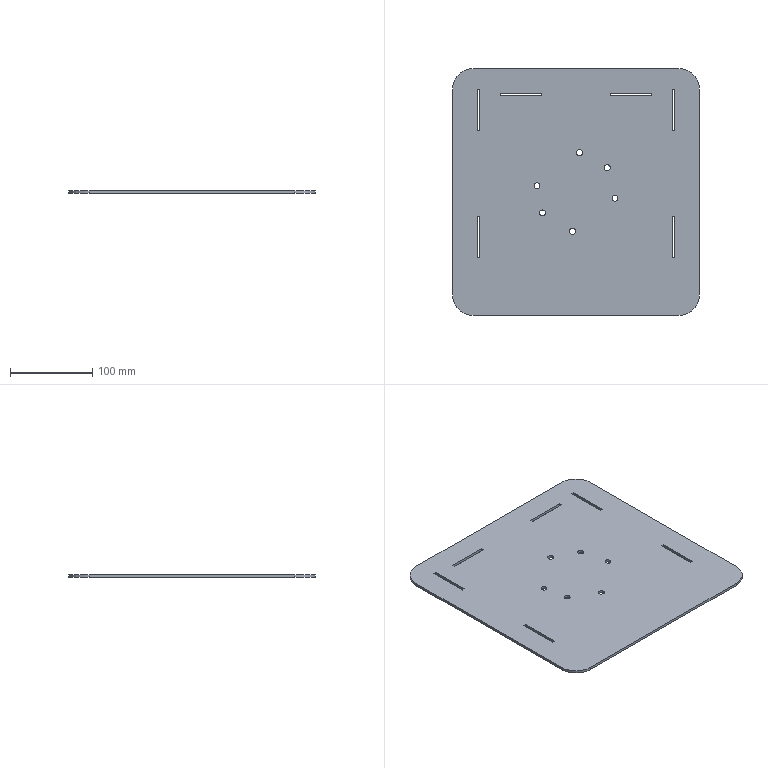Part | SolidWorks | features FlatPattern 1, SMBaseFlange 1, SheetMetal 1 | 1 solid | 46 faces | box 300 x 300 x 3.2 mm | volume 282429 mm3 | plane 30 | cylinder 16 | commonest cylinder face diameters 7.2 x12 50 x4
STEP:
#1=CARTESIAN_POINT('',(-41.465,31.655,3.2));
#2=VERTEX_POINT('',#1);
#3=CARTESIAN_POINT('',(-34.265,31.655,3.2));
#4=VERTEX_POINT('',#3);
#5=CARTESIAN_POINT('',(-37.865,31.655,3.2));
#6=DIRECTION('',(0.,0.,1.));
#7=DIRECTION('',(1.,0.,0.));
#8=AXIS2_PLACEMENT_3D('',#5,#6,#7);
#9=CIRCLE('',#8,3.6);
#10=EDGE_CURVE('',#2,#4,#9,.T.);
#11=ORIENTED_EDGE('',*,*,#10,.T.);
#12=CARTESIAN_POINT('',(-34.265,31.655,0.));
#13=VERTEX_POINT('',#12);
#14=CARTESIAN_POINT('',(-34.265,31.655,3.2));
#15=DIRECTION('',(0.,0.,-1.));
#16=VECTOR('',#15,1000.);
#17=LINE('',#14,#16);
#18=EDGE_CURVE('',#4,#13,#17,.T.);
#19=ORIENTED_EDGE('',*,*,#18,.T.);
#20=CARTESIAN_POINT('',(-41.465,31.655,0.));
#21=VERTEX_POINT('',#20);
#22=CARTESIAN_POINT('',(-37.865,31.655,0.));
#23=DIRECTION('',(0.,0.,1.));
#24=DIRECTION('',(1.,0.,0.));
#25=AXIS2_PLACEMENT_3D('',#22,#23,#24);
#26=CIRCLE('',#25,3.6);
#27=EDGE_CURVE('',#21,#13,#26,.T.);
#28=ORIENTED_EDGE('',*,*,#27,.F.);
#29=CARTESIAN_POINT('',(-41.465,31.655,3.2));
#30=DIRECTION('',(0.,0.,-1.));
#31=VECTOR('',#30,1000.);
#32=LINE('',#29,#31);
#33=EDGE_CURVE('',#2,#21,#32,.T.);
#34=ORIENTED_EDGE('',*,*,#33,.F.);
#35=EDGE_LOOP('',(#11,#19,#28,#34));
#36=FACE_OUTER_BOUND('',#35,.T.);
#37=CARTESIAN_POINT('',(-37.865,31.655,3.2));
#38=DIRECTION('',(0.,0.,-1.));
#39=DIRECTION('',(-1.,0.,0.));
#40=AXIS2_PLACEMENT_3D('',#37,#38,#39);
#41=CYLINDRICAL_SURFACE('',#40,3.6);
#42=ADVANCED_FACE('',(#36),#41,.F.);
#43=CARTESIAN_POINT('',(-34.762,-1.29,3.2));
#44=VERTEX_POINT('',#43);
#45=CARTESIAN_POINT('',(-27.562,-1.29,3.2));
#46=VERTEX_POINT('',#45);
#47=CARTESIAN_POINT('',(-31.162,-1.29,3.2));
#48=DIRECTION('',(0.,0.,1.));
#49=DIRECTION('',(1.,0.,0.));
#50=AXIS2_PLACEMENT_3D('',#47,#48,#49);
#51=CIRCLE('',#50,3.6);
#52=EDGE_CURVE('',#44,#46,#51,.T.);
#53=ORIENTED_EDGE('',*,*,#52,.T.);
#54=CARTESIAN_POINT('',(-27.562,-1.29,0.));
#55=VERTEX_POINT('',#54);
#56=CARTESIAN_POINT('',(-27.562,-1.29,3.2));
#57=DIRECTION('',(0.,0.,-1.));
#58=VECTOR('',#57,1000.);
#59=LINE('',#56,#58);
#60=EDGE_CURVE('',#46,#55,#59,.T.);
#61=ORIENTED_EDGE('',*,*,#60,.T.);
#62=CARTESIAN_POINT('',(-34.762,-1.29,0.));
#63=VERTEX_POINT('',#62);
#64=CARTESIAN_POINT('',(-31.162,-1.29,0.));
#65=DIRECTION('',(0.,0.,1.));
#66=DIRECTION('',(1.,0.,0.));
#67=AXIS2_PLACEMENT_3D('',#64,#65,#66);
#68=CIRCLE('',#67,3.6);
#69=EDGE_CURVE('',#63,#55,#68,.T.);
#70=ORIENTED_EDGE('',*,*,#69,.F.);
#71=CARTESIAN_POINT('',(-34.762,-1.29,3.2));
#72=DIRECTION('',(0.,0.,-1.));
#73=VECTOR('',#72,1000.);
#74=LINE('',#71,#73);
#75=EDGE_CURVE('',#44,#63,#74,.T.);
#76=ORIENTED_EDGE('',*,*,#75,.F.);
#77=EDGE_LOOP('',(#53,#61,#70,#76));
#78=FACE_OUTER_BOUND('',#77,.T.);
#79=CARTESIAN_POINT('',(-31.162,-1.29,3.2));
#80=DIRECTION('',(0.,0.,-1.));
#81=DIRECTION('',(-1.,0.,0.));
#82=AXIS2_PLACEMENT_3D('',#79,#80,#81);
#83=CYLINDRICAL_SURFACE('',#82,3.6);
#84=ADVANCED_FACE('',(#78),#83,.F.);
#85=CARTESIAN_POINT('',(1.761,-23.671,3.2));
#86=VERTEX_POINT('',#85);
#87=CARTESIAN_POINT('',(8.961,-23.671,3.2));
#88=VERTEX_POINT('',#87);
#89=CARTESIAN_POINT('',(5.361,-23.671,3.2));
#90=DIRECTION('',(0.,0.,1.));
#91=DIRECTION('',(1.,0.,0.));
#92=AXIS2_PLACEMENT_3D('',#89,#90,#91);
#93=CIRCLE('',#92,3.6);
#94=EDGE_CURVE('',#86,#88,#93,.T.);
#95=ORIENTED_EDGE('',*,*,#94,.T.);
#96=CARTESIAN_POINT('',(8.961,-23.671,0.));
#97=VERTEX_POINT('',#96);
#98=CARTESIAN_POINT('',(8.961,-23.671,3.2));
#99=DIRECTION('',(0.,0.,-1.));
#100=VECTOR('',#99,1000.);
#101=LINE('',#98,#100);
#102=EDGE_CURVE('',#88,#97,#101,.T.);
#103=ORIENTED_EDGE('',*,*,#102,.T.);
#104=CARTESIAN_POINT('',(1.761,-23.671,0.));
#105=VERTEX_POINT('',#104);
#106=CARTESIAN_POINT('',(5.361,-23.671,0.));
#107=DIRECTION('',(0.,0.,1.));
#108=DIRECTION('',(1.,0.,0.));
#109=AXIS2_PLACEMENT_3D('',#106,#107,#108);
#110=CIRCLE('',#109,3.6);
#111=EDGE_CURVE('',#105,#97,#110,.T.);
#112=ORIENTED_EDGE('',*,*,#111,.F.);
#113=CARTESIAN_POINT('',(1.761,-23.671,3.2));
#114=DIRECTION('',(0.,0.,-1.));
#115=VECTOR('',#114,1000.);
#116=LINE('',#113,#115);
#117=EDGE_CURVE('',#86,#105,#116,.T.);
#118=ORIENTED_EDGE('',*,*,#117,.F.);
#119=EDGE_LOOP('',(#95,#103,#112,#118));
#120=FACE_OUTER_BOUND('',#119,.T.);
#121=CARTESIAN_POINT('',(5.361,-23.671,3.2));
#122=DIRECTION('',(0.,0.,-1.));
#123=DIRECTION('',(-1.,0.,0.));
#124=AXIS2_PLACEMENT_3D('',#121,#122,#123);
#125=CYLINDRICAL_SURFACE('',#124,3.6);
#126=ADVANCED_FACE('',(#120),#125,.F.);
#127=CARTESIAN_POINT('',(53.354,16.637,3.2));
#128=VERTEX_POINT('',#127);
#129=CARTESIAN_POINT('',(60.554,16.637,3.2));
#130=VERTEX_POINT('',#129);
#131=CARTESIAN_POINT('',(56.954,16.637,3.2));
#132=DIRECTION('',(0.,0.,1.));
#133=DIRECTION('',(1.,0.,0.));
#134=AXIS2_PLACEMENT_3D('',#131,#132,#133);
#135=CIRCLE('',#134,3.6);
#136=EDGE_CURVE('',#128,#130,#135,.T.);
#137=ORIENTED_EDGE('',*,*,#136,.T.);
#138=CARTESIAN_POINT('',(60.554,16.637,0.));
#139=VERTEX_POINT('',#138);
#140=CARTESIAN_POINT('',(60.554,16.637,3.2));
#141=DIRECTION('',(0.,0.,-1.));
#142=VECTOR('',#141,1000.);
#143=LINE('',#140,#142);
#144=EDGE_CURVE('',#130,#139,#143,.T.);
#145=ORIENTED_EDGE('',*,*,#144,.T.);
#146=CARTESIAN_POINT('',(53.354,16.637,0.));
#147=VERTEX_POINT('',#146);
#148=CARTESIAN_POINT('',(56.954,16.637,0.));
#149=DIRECTION('',(0.,0.,1.));
#150=DIRECTION('',(1.,0.,0.));
#151=AXIS2_PLACEMENT_3D('',#148,#149,#150);
#152=CIRCLE('',#151,3.6);
#153=EDGE_CURVE('',#147,#139,#152,.T.);
#154=ORIENTED_EDGE('',*,*,#153,.F.);
#155=CARTESIAN_POINT('',(53.354,16.637,3.2));
#156=DIRECTION('',(0.,0.,-1.));
#157=VECTOR('',#156,1000.);
#158=LINE('',#155,#157);
#159=EDGE_CURVE('',#128,#147,#158,.T.);
#160=ORIENTED_EDGE('',*,*,#159,.F.);
#161=EDGE_LOOP('',(#137,#145,#154,#160));
#162=FACE_OUTER_BOUND('',#161,.T.);
#163=CARTESIAN_POINT('',(56.954,16.637,3.2));
#164=DIRECTION('',(0.,0.,-1.));
#165=DIRECTION('',(-1.,0.,0.));
#166=AXIS2_PLACEMENT_3D('',#163,#164,#165);
#167=CYLINDRICAL_SURFACE('',#166,3.6);
#168=ADVANCED_FACE('',(#162),#167,.F.);
#169=CARTESIAN_POINT('',(43.769,53.698,3.2));
#170=VERTEX_POINT('',#169);
#171=CARTESIAN_POINT('',(50.969,53.698,3.2));
#172=VERTEX_POINT('',#171);
#173=CARTESIAN_POINT('',(47.369,53.698,3.2));
#174=DIRECTION('',(0.,0.,1.));
#175=DIRECTION('',(1.,0.,0.));
#176=AXIS2_PLACEMENT_3D('',#173,#174,#175);
#177=CIRCLE('',#176,3.6);
#178=EDGE_CURVE('',#170,#172,#177,.T.);
#179=ORIENTED_EDGE('',*,*,#178,.T.);
#180=CARTESIAN_POINT('',(50.969,53.698,0.));
#181=VERTEX_POINT('',#180);
#182=CARTESIAN_POINT('',(50.969,53.698,3.2));
#183=DIRECTION('',(0.,0.,-1.));
#184=VECTOR('',#183,1000.);
#185=LINE('',#182,#184);
#186=EDGE_CURVE('',#172,#181,#185,.T.);
#187=ORIENTED_EDGE('',*,*,#186,.T.);
#188=CARTESIAN_POINT('',(43.769,53.698,0.));
#189=VERTEX_POINT('',#188);
#190=CARTESIAN_POINT('',(47.369,53.698,0.));
#191=DIRECTION('',(0.,0.,1.));
#192=DIRECTION('',(1.,0.,0.));
#193=AXIS2_PLACEMENT_3D('',#190,#191,#192);
#194=CIRCLE('',#193,3.6);
#195=EDGE_CURVE('',#189,#181,#194,.T.);
#196=ORIENTED_EDGE('',*,*,#195,.F.);
#197=CARTESIAN_POINT('',(43.769,53.698,3.2));
#198=DIRECTION('',(0.,0.,-1.));
#199=VECTOR('',#198,1000.);
#200=LINE('',#197,#199);
#201=EDGE_CURVE('',#170,#189,#200,.T.);
#202=ORIENTED_EDGE('',*,*,#201,.F.);
#203=EDGE_LOOP('',(#179,#187,#196,#202));
#204=FACE_OUTER_BOUND('',#203,.T.);
#205=CARTESIAN_POINT('',(47.369,53.698,3.2));
#206=DIRECTION('',(0.,0.,-1.));
#207=DIRECTION('',(-1.,0.,0.));
#208=AXIS2_PLACEMENT_3D('',#205,#206,#207);
#209=CYLINDRICAL_SURFACE('',#208,3.6);
#210=ADVANCED_FACE('',(#204),#209,.F.);
#211=CARTESIAN_POINT('',(10.128,71.964,3.2));
#212=VERTEX_POINT('',#211);
#213=CARTESIAN_POINT('',(17.328,71.964,3.2));
#214=VERTEX_POINT('',#213);
#215=CARTESIAN_POINT('',(13.728,71.964,3.2));
#216=DIRECTION('',(0.,0.,1.));
#217=DIRECTION('',(1.,0.,0.));
#218=AXIS2_PLACEMENT_3D('',#215,#216,#217);
#219=CIRCLE('',#218,3.6);
#220=EDGE_CURVE('',#212,#214,#219,.T.);
#221=ORIENTED_EDGE('',*,*,#220,.T.);
#222=CARTESIAN_POINT('',(17.328,71.964,0.));
#223=VERTEX_POINT('',#222);
#224=CARTESIAN_POINT('',(17.328,71.964,3.2));
#225=DIRECTION('',(0.,0.,-1.));
#226=VECTOR('',#225,1000.);
#227=LINE('',#224,#226);
#228=EDGE_CURVE('',#214,#223,#227,.T.);
#229=ORIENTED_EDGE('',*,*,#228,.T.);
#230=CARTESIAN_POINT('',(10.128,71.964,0.));
#231=VERTEX_POINT('',#230);
#232=CARTESIAN_POINT('',(13.728,71.964,0.));
#233=DIRECTION('',(0.,0.,1.));
#234=DIRECTION('',(1.,0.,0.));
#235=AXIS2_PLACEMENT_3D('',#232,#233,#234);
#236=CIRCLE('',#235,3.6);
#237=EDGE_CURVE('',#231,#223,#236,.T.);
#238=ORIENTED_EDGE('',*,*,#237,.F.);
#239=CARTESIAN_POINT('',(10.128,71.964,3.2));
#240=DIRECTION('',(0.,0.,-1.));
#241=VECTOR('',#240,1000.);
#242=LINE('',#239,#241);
#243=EDGE_CURVE('',#212,#231,#242,.T.);
#244=ORIENTED_EDGE('',*,*,#243,.F.);
#245=EDGE_LOOP('',(#221,#229,#238,#244));
#246=FACE_OUTER_BOUND('',#245,.T.);
#247=CARTESIAN_POINT('',(13.728,71.964,3.2));
#248=DIRECTION('',(0.,0.,-1.));
#249=DIRECTION('',(-1.,0.,0.));
#250=AXIS2_PLACEMENT_3D('',#247,#248,#249);
#251=CYLINDRICAL_SURFACE('',#250,3.6);
#252=ADVANCED_FACE('',(#246),#251,.F.);
#253=ORIENTED_EDGE('',*,*,#52,.F.);
#254=CARTESIAN_POINT('',(-31.162,-1.29,3.2));
#255=DIRECTION('',(0.,0.,1.));
#256=DIRECTION('',(1.,0.,0.));
#257=AXIS2_PLACEMENT_3D('',#254,#255,#256);
#258=CIRCLE('',#257,3.6);
#259=EDGE_CURVE('',#46,#44,#258,.T.);
#260=ORIENTED_EDGE('',*,*,#259,.F.);
#261=EDGE_LOOP('',(#253,#260));
#262=FACE_BOUND('',#261,.T.);
#263=ORIENTED_EDGE('',*,*,#136,.F.);
#264=CARTESIAN_POINT('',(56.954,16.637,3.2));
#265=DIRECTION('',(0.,0.,1.));
#266=DIRECTION('',(1.,0.,0.));
#267=AXIS2_PLACEMENT_3D('',#264,#265,#266);
#268=CIRCLE('',#267,3.6);
#269=EDGE_CURVE('',#130,#128,#268,.T.);
#270=ORIENTED_EDGE('',*,*,#269,.F.);
#271=EDGE_LOOP('',(#263,#270));
#272=FACE_BOUND('',#271,.T.);
#273=ORIENTED_EDGE('',*,*,#220,.F.);
#274=CARTESIAN_POINT('',(13.728,71.964,3.2));
#275=DIRECTION('',(0.,0.,1.));
#276=DIRECTION('',(1.,0.,0.));
#277=AXIS2_PLACEMENT_3D('',#274,#275,#276);
#278=CIRCLE('',#277,3.6);
#279=EDGE_CURVE('',#214,#212,#278,.T.);
#280=ORIENTED_EDGE('',*,*,#279,.F.);
#281=EDGE_LOOP('',(#273,#280));
#282=FACE_BOUND('',#281,.T.);
#283=CARTESIAN_POINT('',(-140.456,-100.854,3.2));
#284=VERTEX_POINT('',#283);
#285=CARTESIAN_POINT('',(-115.456,-125.854,3.2));
#286=VERTEX_POINT('',#285);
#287=CARTESIAN_POINT('',(-115.456,-100.854,3.2));
#288=DIRECTION('',(0.,0.,1.));
#289=DIRECTION('',(1.,0.,0.));
#290=AXIS2_PLACEMENT_3D('',#287,#288,#289);
#291=CIRCLE('',#290,25.);
#292=EDGE_CURVE('',#284,#286,#291,.T.);
#293=ORIENTED_EDGE('',*,*,#292,.T.);
#294=CARTESIAN_POINT('',(134.544,-125.854,3.2));
#295=VERTEX_POINT('',#294);
#296=CARTESIAN_POINT('',(-115.456,-125.854,3.2));
#297=DIRECTION('',(1.,0.,0.));
#298=VECTOR('',#297,1000.);
#299=LINE('',#296,#298);
#300=EDGE_CURVE('',#286,#295,#299,.T.);
#301=ORIENTED_EDGE('',*,*,#300,.T.);
#302=CARTESIAN_POINT('',(159.544,-100.854,3.2));
#303=VERTEX_POINT('',#302);
#304=CARTESIAN_POINT('',(134.544,-100.854,3.2));
#305=DIRECTION('',(0.,0.,1.));
#306=DIRECTION('',(1.,0.,0.));
#307=AXIS2_PLACEMENT_3D('',#304,#305,#306);
#308=CIRCLE('',#307,25.);
#309=EDGE_CURVE('',#295,#303,#308,.T.);
#310=ORIENTED_EDGE('',*,*,#309,.T.);
#311=CARTESIAN_POINT('',(159.544,149.146,3.2));
#312=VERTEX_POINT('',#311);
#313=CARTESIAN_POINT('',(159.544,149.146,3.2));
#314=DIRECTION('',(0.,1.,0.));
#315=VECTOR('',#314,1000.);
#316=LINE('',#313,#315);
#317=EDGE_CURVE('',#303,#312,#316,.T.);
#318=ORIENTED_EDGE('',*,*,#317,.T.);
#319=CARTESIAN_POINT('',(134.544,174.146,3.2));
#320=VERTEX_POINT('',#319);
#321=CARTESIAN_POINT('',(134.544,149.146,3.2));
#322=DIRECTION('',(0.,0.,1.));
#323=DIRECTION('',(-1.,0.,0.));
#324=AXIS2_PLACEMENT_3D('',#321,#322,#323);
#325=CIRCLE('',#324,25.);
#326=EDGE_CURVE('',#312,#320,#325,.T.);
#327=ORIENTED_EDGE('',*,*,#326,.T.);
#328=CARTESIAN_POINT('',(-115.456,174.146,3.2));
#329=VERTEX_POINT('',#328);
#330=CARTESIAN_POINT('',(-115.456,174.146,3.2));
#331=DIRECTION('',(-1.,0.,0.));
#332=VECTOR('',#331,1000.);
#333=LINE('',#330,#332);
#334=EDGE_CURVE('',#320,#329,#333,.T.);
#335=ORIENTED_EDGE('',*,*,#334,.T.);
#336=CARTESIAN_POINT('',(-140.456,149.146,3.2));
#337=VERTEX_POINT('',#336);
#338=CARTESIAN_POINT('',(-115.456,149.146,3.2));
#339=DIRECTION('',(0.,0.,1.));
#340=DIRECTION('',(1.,0.,0.));
#341=AXIS2_PLACEMENT_3D('',#338,#339,#340);
#342=CIRCLE('',#341,25.);
#343=EDGE_CURVE('',#329,#337,#342,.T.);
#344=ORIENTED_EDGE('',*,*,#343,.T.);
#345=CARTESIAN_POINT('',(-140.456,149.146,3.2));
#346=DIRECTION('',(0.,-1.,0.));
#347=VECTOR('',#346,1000.);
#348=LINE('',#345,#347);
#349=EDGE_CURVE('',#337,#284,#348,.T.);
#350=ORIENTED_EDGE('',*,*,#349,.T.);
#351=EDGE_LOOP('',(#293,#301,#310,#318,#327,#335,#344,#350));
#352=FACE_OUTER_BOUND('',#351,.T.);
#353=ORIENTED_EDGE('',*,*,#178,.F.);
#354=CARTESIAN_POINT('',(47.369,53.698,3.2));
#355=DIRECTION('',(0.,0.,1.));
#356=DIRECTION('',(1.,0.,0.));
#357=AXIS2_PLACEMENT_3D('',#354,#355,#356);
#358=CIRCLE('',#357,3.6);
#359=EDGE_CURVE('',#172,#170,#358,.T.);
#360=ORIENTED_EDGE('',*,*,#359,.F.);
#361=EDGE_LOOP('',(#353,#360));
#362=FACE_BOUND('',#361,.T.);
#363=ORIENTED_EDGE('',*,*,#94,.F.);
#364=CARTESIAN_POINT('',(5.361,-23.671,3.2));
#365=DIRECTION('',(0.,0.,1.));
#366=DIRECTION('',(1.,0.,0.));
#367=AXIS2_PLACEMENT_3D('',#364,#365,#366);
#368=CIRCLE('',#367,3.6);
#369=EDGE_CURVE('',#88,#86,#368,.T.);
#370=ORIENTED_EDGE('',*,*,#369,.F.);
#371=EDGE_LOOP('',(#363,#370));
#372=FACE_BOUND('',#371,.T.);
#373=ORIENTED_EDGE('',*,*,#10,.F.);
#374=CARTESIAN_POINT('',(-37.865,31.655,3.2));
#375=DIRECTION('',(0.,0.,1.));
#376=DIRECTION('',(1.,0.,0.));
#377=AXIS2_PLACEMENT_3D('',#374,#375,#376);
#378=CIRCLE('',#377,3.6);
#379=EDGE_CURVE('',#4,#2,#378,.T.);
#380=ORIENTED_EDGE('',*,*,#379,.F.);
#381=EDGE_LOOP('',(#373,#380));
#382=FACE_BOUND('',#381,.T.);
#383=CARTESIAN_POINT('',(126.344,-55.854,3.2));
#384=VERTEX_POINT('',#383);
#385=CARTESIAN_POINT('',(129.544,-55.854,3.2));
#386=VERTEX_POINT('',#385);
#387=CARTESIAN_POINT('',(126.344,-55.854,3.2));
#388=DIRECTION('',(1.,0.,0.));
#389=VECTOR('',#388,1000.);
#390=LINE('',#387,#389);
#391=EDGE_CURVE('',#384,#386,#390,.T.);
#392=ORIENTED_EDGE('',*,*,#391,.F.);
#393=CARTESIAN_POINT('',(126.344,-5.854,3.2));
#394=VERTEX_POINT('',#393);
#395=CARTESIAN_POINT('',(126.344,-55.854,3.2));
#396=DIRECTION('',(0.,-1.,0.));
#397=VECTOR('',#396,1000.);
#398=LINE('',#395,#397);
#399=EDGE_CURVE('',#394,#384,#398,.T.);
#400=ORIENTED_EDGE('',*,*,#399,.F.);
#401=CARTESIAN_POINT('',(129.544,-5.854,3.2));
#402=VERTEX_POINT('',#401);
#403=CARTESIAN_POINT('',(126.344,-5.854,3.2));
#404=DIRECTION('',(-1.,0.,0.));
#405=VECTOR('',#404,1000.);
#406=LINE('',#403,#405);
#407=EDGE_CURVE('',#402,#394,#406,.T.);
#408=ORIENTED_EDGE('',*,*,#407,.F.);
#409=CARTESIAN_POINT('',(129.544,-55.854,3.2));
#410=DIRECTION('',(0.,1.,0.));
#411=VECTOR('',#410,1000.);
#412=LINE('',#409,#411);
#413=EDGE_CURVE('',#386,#402,#412,.T.);
#414=ORIENTED_EDGE('',*,*,#413,.F.);
#415=EDGE_LOOP('',(#392,#400,#408,#414));
#416=FACE_BOUND('',#415,.T.);
#417=CARTESIAN_POINT('',(126.344,99.146,3.2));
#418=VERTEX_POINT('',#417);
#419=CARTESIAN_POINT('',(129.544,99.146,3.2));
#420=VERTEX_POINT('',#419);
#421=CARTESIAN_POINT('',(126.344,99.146,3.2));
#422=DIRECTION('',(1.,0.,0.));
#423=VECTOR('',#422,1000.);
#424=LINE('',#421,#423);
#425=EDGE_CURVE('',#418,#420,#424,.T.);
#426=ORIENTED_EDGE('',*,*,#425,.F.);
#427=CARTESIAN_POINT('',(126.344,149.146,3.2));
#428=VERTEX_POINT('',#427);
#429=CARTESIAN_POINT('',(126.344,99.146,3.2));
#430=DIRECTION('',(0.,-1.,0.));
#431=VECTOR('',#430,1000.);
#432=LINE('',#429,#431);
#433=EDGE_CURVE('',#428,#418,#432,.T.);
#434=ORIENTED_EDGE('',*,*,#433,.F.);
#435=CARTESIAN_POINT('',(129.544,149.146,3.2));
#436=VERTEX_POINT('',#435);
#437=CARTESIAN_POINT('',(126.344,149.146,3.2));
#438=DIRECTION('',(-1.,0.,0.));
#439=VECTOR('',#438,1000.);
#440=LINE('',#437,#439);
#441=EDGE_CURVE('',#436,#428,#440,.T.);
#442=ORIENTED_EDGE('',*,*,#441,.F.);
#443=CARTESIAN_POINT('',(129.544,99.146,3.2));
#444=DIRECTION('',(0.,1.,0.));
#445=VECTOR('',#444,1000.);
#446=LINE('',#443,#445);
#447=EDGE_CURVE('',#420,#436,#446,.T.);
#448=ORIENTED_EDGE('',*,*,#447,.F.);
#449=EDGE_LOOP('',(#426,#434,#442,#448));
#450=FACE_BOUND('',#449,.T.);
#451=CARTESIAN_POINT('',(101.344,144.146,3.2));
#452=VERTEX_POINT('',#451);
#453=CARTESIAN_POINT('',(51.344,144.146,3.2));
#454=VERTEX_POINT('',#453);
#455=CARTESIAN_POINT('',(101.344,144.146,3.2));
#456=DIRECTION('',(-1.,0.,0.));
#457=VECTOR('',#456,1000.);
#458=LINE('',#455,#457);
#459=EDGE_CURVE('',#452,#454,#458,.T.);
#460=ORIENTED_EDGE('',*,*,#459,.F.);
#461=CARTESIAN_POINT('',(101.344,140.946,3.2));
#462=VERTEX_POINT('',#461);
#463=CARTESIAN_POINT('',(101.344,144.146,3.2));
#464=DIRECTION('',(0.,1.,0.));
#465=VECTOR('',#464,1000.);
#466=LINE('',#463,#465);
#467=EDGE_CURVE('',#462,#452,#466,.T.);
#468=ORIENTED_EDGE('',*,*,#467,.F.);
#469=CARTESIAN_POINT('',(51.344,140.946,3.2));
#470=VERTEX_POINT('',#469);
#471=CARTESIAN_POINT('',(101.344,140.946,3.2));
#472=DIRECTION('',(1.,0.,0.));
#473=VECTOR('',#472,1000.);
#474=LINE('',#471,#473);
#475=EDGE_CURVE('',#470,#462,#474,.T.);
#476=ORIENTED_EDGE('',*,*,#475,.F.);
#477=CARTESIAN_POINT('',(51.344,144.146,3.2));
#478=DIRECTION('',(0.,-1.,0.));
#479=VECTOR('',#478,1000.);
#480=LINE('',#477,#479);
#481=EDGE_CURVE('',#454,#470,#480,.T.);
#482=ORIENTED_EDGE('',*,*,#481,.F.);
#483=EDGE_LOOP('',(#460,#468,#476,#482));
#484=FACE_BOUND('',#483,.T.);
#485=CARTESIAN_POINT('',(-82.256,140.946,3.2));
#486=VERTEX_POINT('',#485);
#487=CARTESIAN_POINT('',(-32.256,140.946,3.2));
#488=VERTEX_POINT('',#487);
#489=CARTESIAN_POINT('',(-82.256,140.946,3.2));
#490=DIRECTION('',(1.,0.,0.));
#491=VECTOR('',#490,1000.);
#492=LINE('',#489,#491);
#493=EDGE_CURVE('',#486,#488,#492,.T.);
#494=ORIENTED_EDGE('',*,*,#493,.F.);
#495=CARTESIAN_POINT('',(-82.256,144.146,3.2));
#496=VERTEX_POINT('',#495);
#497=CARTESIAN_POINT('',(-82.256,140.946,3.2));
#498=DIRECTION('',(0.,-1.,0.));
#499=VECTOR('',#498,1000.);
#500=LINE('',#497,#499);
#501=EDGE_CURVE('',#496,#486,#500,.T.);
#502=ORIENTED_EDGE('',*,*,#501,.F.);
#503=CARTESIAN_POINT('',(-32.256,144.146,3.2));
#504=VERTEX_POINT('',#503);
#505=CARTESIAN_POINT('',(-82.256,144.146,3.2));
#506=DIRECTION('',(-1.,0.,0.));
#507=VECTOR('',#506,1000.);
#508=LINE('',#505,#507);
#509=EDGE_CURVE('',#504,#496,#508,.T.);
#510=ORIENTED_EDGE('',*,*,#509,.F.);
#511=CARTESIAN_POINT('',(-32.256,140.946,3.2));
#512=DIRECTION('',(0.,1.,0.));
#513=VECTOR('',#512,1000.);
#514=LINE('',#511,#513);
#515=EDGE_CURVE('',#488,#504,#514,.T.);
#516=ORIENTED_EDGE('',*,*,#515,.F.);
#517=EDGE_LOOP('',(#494,#502,#510,#516));
#518=FACE_BOUND('',#517,.T.);
#519=CARTESIAN_POINT('',(-110.456,99.146,3.2));
#520=VERTEX_POINT('',#519);
#521=CARTESIAN_POINT('',(-107.256,99.146,3.2));
#522=VERTEX_POINT('',#521);
#523=CARTESIAN_POINT('',(-110.456,99.146,3.2));
#524=DIRECTION('',(1.,0.,0.));
#525=VECTOR('',#524,1000.);
#526=LINE('',#523,#525);
#527=EDGE_CURVE('',#520,#522,#526,.T.);
#528=ORIENTED_EDGE('',*,*,#527,.F.);
#529=CARTESIAN_POINT('',(-110.456,149.146,3.2));
#530=VERTEX_POINT('',#529);
#531=CARTESIAN_POINT('',(-110.456,149.146,3.2));
#532=DIRECTION('',(0.,-1.,0.));
#533=VECTOR('',#532,1000.);
#534=LINE('',#531,#533);
#535=EDGE_CURVE('',#530,#520,#534,.T.);
#536=ORIENTED_EDGE('',*,*,#535,.F.);
#537=CARTESIAN_POINT('',(-107.256,149.146,3.2));
#538=VERTEX_POINT('',#537);
#539=CARTESIAN_POINT('',(-110.456,149.146,3.2));
#540=DIRECTION('',(-1.,0.,0.));
#541=VECTOR('',#540,1000.);
#542=LINE('',#539,#541);
#543=EDGE_CURVE('',#538,#530,#542,.T.);
#544=ORIENTED_EDGE('',*,*,#543,.F.);
#545=CARTESIAN_POINT('',(-107.256,149.146,3.2));
#546=DIRECTION('',(0.,1.,0.));
#547=VECTOR('',#546,1000.);
#548=LINE('',#545,#547);
#549=EDGE_CURVE('',#522,#538,#548,.T.);
#550=ORIENTED_EDGE('',*,*,#549,.F.);
#551=EDGE_LOOP('',(#528,#536,#544,#550));
#552=FACE_BOUND('',#551,.T.);
#553=CARTESIAN_POINT('',(-110.456,-55.854,3.2));
#554=VERTEX_POINT('',#553);
#555=CARTESIAN_POINT('',(-107.256,-55.854,3.2));
#556=VERTEX_POINT('',#555);
#557=CARTESIAN_POINT('',(-110.456,-55.854,3.2));
#558=DIRECTION('',(1.,0.,0.));
#559=VECTOR('',#558,1000.);
#560=LINE('',#557,#559);
#561=EDGE_CURVE('',#554,#556,#560,.T.);
#562=ORIENTED_EDGE('',*,*,#561,.F.);
#563=CARTESIAN_POINT('',(-110.456,-5.854,3.2));
#564=VERTEX_POINT('',#563);
#565=CARTESIAN_POINT('',(-110.456,-55.854,3.2));
#566=DIRECTION('',(0.,-1.,0.));
#567=VECTOR('',#566,1000.);
#568=LINE('',#565,#567);
#569=EDGE_CURVE('',#564,#554,#568,.T.);
#570=ORIENTED_EDGE('',*,*,#569,.F.);
#571=CARTESIAN_POINT('',(-107.256,-5.854,3.2));
#572=VERTEX_POINT('',#571);
#573=CARTESIAN_POINT('',(-110.456,-5.854,3.2));
#574=DIRECTION('',(-1.,0.,0.));
#575=VECTOR('',#574,1000.);
#576=LINE('',#573,#575);
#577=EDGE_CURVE('',#572,#564,#576,.T.);
#578=ORIENTED_EDGE('',*,*,#577,.F.);
#579=CARTESIAN_POINT('',(-107.256,-55.854,3.2));
#580=DIRECTION('',(0.,1.,0.));
#581=VECTOR('',#580,1000.);
#582=LINE('',#579,#581);
#583=EDGE_CURVE('',#556,#572,#582,.T.);
#584=ORIENTED_EDGE('',*,*,#583,.F.);
#585=EDGE_LOOP('',(#562,#570,#578,#584));
#586=FACE_BOUND('',#585,.T.);
#587=CARTESIAN_POINT('',(-115.456,-100.854,3.2));
#588=DIRECTION('',(0.,0.,1.));
#589=DIRECTION('',(1.,0.,0.));
#590=AXIS2_PLACEMENT_3D('',#587,#588,#589);
#591=PLANE('',#590);
#592=ADVANCED_FACE('',(#262,#272,#282,#352,#362,#372,#382,#416,#450,#484,#518,#552,#586),#591,.T.);
#593=CARTESIAN_POINT('',(-110.456,149.146,0.));
#594=VERTEX_POINT('',#593);
#595=CARTESIAN_POINT('',(-110.456,99.146,0.));
#596=VERTEX_POINT('',#595);
#597=CARTESIAN_POINT('',(-110.456,149.146,0.));
#598=DIRECTION('',(0.,-1.,0.));
#599=VECTOR('',#598,1000.);
#600=LINE('',#597,#599);
#601=EDGE_CURVE('',#594,#596,#600,.T.);
#602=ORIENTED_EDGE('',*,*,#601,.T.);
#603=CARTESIAN_POINT('',(-107.256,99.146,0.));
#604=VERTEX_POINT('',#603);
#605=CARTESIAN_POINT('',(-110.456,99.146,0.));
#606=DIRECTION('',(1.,0.,0.));
#607=VECTOR('',#606,1000.);
#608=LINE('',#605,#607);
#609=EDGE_CURVE('',#596,#604,#608,.T.);
#610=ORIENTED_EDGE('',*,*,#609,.T.);
#611=CARTESIAN_POINT('',(-107.256,149.146,0.));
#612=VERTEX_POINT('',#611);
#613=CARTESIAN_POINT('',(-107.256,149.146,0.));
#614=DIRECTION('',(0.,1.,0.));
#615=VECTOR('',#614,1000.);
#616=LINE('',#613,#615);
#617=EDGE_CURVE('',#604,#612,#616,.T.);
#618=ORIENTED_EDGE('',*,*,#617,.T.);
#619=CARTESIAN_POINT('',(-110.456,149.146,0.));
#620=DIRECTION('',(-1.,0.,0.));
#621=VECTOR('',#620,1000.);
#622=LINE('',#619,#621);
#623=EDGE_CURVE('',#612,#594,#622,.T.);
#624=ORIENTED_EDGE('',*,*,#623,.T.);
#625=EDGE_LOOP('',(#602,#610,#618,#624));
#626=FACE_BOUND('',#625,.T.);
#627=CARTESIAN_POINT('',(101.344,140.946,0.));
#628=VERTEX_POINT('',#627);
#629=CARTESIAN_POINT('',(101.344,144.146,0.));
#630=VERTEX_POINT('',#629);
#631=CARTESIAN_POINT('',(101.344,144.146,0.));
#632=DIRECTION('',(0.,1.,0.));
#633=VECTOR('',#632,1000.);
#634=LINE('',#631,#633);
#635=EDGE_CURVE('',#628,#630,#634,.T.);
#636=ORIENTED_EDGE('',*,*,#635,.T.);
#637=CARTESIAN_POINT('',(51.344,144.146,0.));
#638=VERTEX_POINT('',#637);
#639=CARTESIAN_POINT('',(101.344,144.146,0.));
#640=DIRECTION('',(-1.,0.,0.));
#641=VECTOR('',#640,1000.);
#642=LINE('',#639,#641);
#643=EDGE_CURVE('',#630,#638,#642,.T.);
#644=ORIENTED_EDGE('',*,*,#643,.T.);
#645=CARTESIAN_POINT('',(51.344,140.946,0.));
#646=VERTEX_POINT('',#645);
#647=CARTESIAN_POINT('',(51.344,144.146,0.));
#648=DIRECTION('',(0.,-1.,0.));
#649=VECTOR('',#648,1000.);
#650=LINE('',#647,#649);
#651=EDGE_CURVE('',#638,#646,#650,.T.);
#652=ORIENTED_EDGE('',*,*,#651,.T.);
#653=CARTESIAN_POINT('',(101.344,140.946,0.));
#654=DIRECTION('',(1.,0.,0.));
#655=VECTOR('',#654,1000.);
#656=LINE('',#653,#655);
#657=EDGE_CURVE('',#646,#628,#656,.T.);
#658=ORIENTED_EDGE('',*,*,#657,.T.);
#659=EDGE_LOOP('',(#636,#644,#652,#658));
#660=FACE_BOUND('',#659,.T.);
#661=CARTESIAN_POINT('',(126.344,-5.854,0.));
#662=VERTEX_POINT('',#661);
#663=CARTESIAN_POINT('',(126.344,-55.854,0.));
#664=VERTEX_POINT('',#663);
#665=CARTESIAN_POINT('',(126.344,-55.854,0.));
#666=DIRECTION('',(0.,-1.,0.));
#667=VECTOR('',#666,1000.);
#668=LINE('',#665,#667);
#669=EDGE_CURVE('',#662,#664,#668,.T.);
#670=ORIENTED_EDGE('',*,*,#669,.T.);
#671=CARTESIAN_POINT('',(129.544,-55.854,0.));
#672=VERTEX_POINT('',#671);
#673=CARTESIAN_POINT('',(126.344,-55.854,0.));
#674=DIRECTION('',(1.,0.,0.));
#675=VECTOR('',#674,1000.);
#676=LINE('',#673,#675);
#677=EDGE_CURVE('',#664,#672,#676,.T.);
#678=ORIENTED_EDGE('',*,*,#677,.T.);
#679=CARTESIAN_POINT('',(129.544,-5.854,0.));
#680=VERTEX_POINT('',#679);
#681=CARTESIAN_POINT('',(129.544,-55.854,0.));
#682=DIRECTION('',(0.,1.,0.));
#683=VECTOR('',#682,1000.);
#684=LINE('',#681,#683);
#685=EDGE_CURVE('',#672,#680,#684,.T.);
#686=ORIENTED_EDGE('',*,*,#685,.T.);
#687=CARTESIAN_POINT('',(126.344,-5.854,0.));
#688=DIRECTION('',(-1.,0.,0.));
#689=VECTOR('',#688,1000.);
#690=LINE('',#687,#689);
#691=EDGE_CURVE('',#680,#662,#690,.T.);
#692=ORIENTED_EDGE('',*,*,#691,.T.);
#693=EDGE_LOOP('',(#670,#678,#686,#692));
#694=FACE_BOUND('',#693,.T.);
#695=CARTESIAN_POINT('',(-140.456,-100.854,0.));
#696=VERTEX_POINT('',#695);
#697=CARTESIAN_POINT('',(-115.456,-125.854,0.));
#698=VERTEX_POINT('',#697);
#699=CARTESIAN_POINT('',(-115.456,-100.854,0.));
#700=DIRECTION('',(0.,0.,1.));
#701=DIRECTION('',(1.,0.,0.));
#702=AXIS2_PLACEMENT_3D('',#699,#700,#701);
#703=CIRCLE('',#702,25.);
#704=EDGE_CURVE('',#696,#698,#703,.T.);
#705=ORIENTED_EDGE('',*,*,#704,.F.);
#706=CARTESIAN_POINT('',(-140.456,149.146,0.));
#707=VERTEX_POINT('',#706);
#708=CARTESIAN_POINT('',(-140.456,149.146,0.));
#709=DIRECTION('',(0.,-1.,0.));
#710=VECTOR('',#709,1000.);
#711=LINE('',#708,#710);
#712=EDGE_CURVE('',#707,#696,#711,.T.);
#713=ORIENTED_EDGE('',*,*,#712,.F.);
#714=CARTESIAN_POINT('',(-115.456,174.146,0.));
#715=VERTEX_POINT('',#714);
#716=CARTESIAN_POINT('',(-115.456,149.146,0.));
#717=DIRECTION('',(0.,0.,1.));
#718=DIRECTION('',(1.,0.,0.));
#719=AXIS2_PLACEMENT_3D('',#716,#717,#718);
#720=CIRCLE('',#719,25.);
#721=EDGE_CURVE('',#715,#707,#720,.T.);
#722=ORIENTED_EDGE('',*,*,#721,.F.);
#723=CARTESIAN_POINT('',(134.544,174.146,0.));
#724=VERTEX_POINT('',#723);
#725=CARTESIAN_POINT('',(-115.456,174.146,0.));
#726=DIRECTION('',(-1.,0.,0.));
#727=VECTOR('',#726,1000.);
#728=LINE('',#725,#727);
#729=EDGE_CURVE('',#724,#715,#728,.T.);
#730=ORIENTED_EDGE('',*,*,#729,.F.);
#731=CARTESIAN_POINT('',(159.544,149.146,0.));
#732=VERTEX_POINT('',#731);
#733=CARTESIAN_POINT('',(134.544,149.146,0.));
#734=DIRECTION('',(0.,0.,1.));
#735=DIRECTION('',(-1.,0.,0.));
#736=AXIS2_PLACEMENT_3D('',#733,#734,#735);
#737=CIRCLE('',#736,25.);
#738=EDGE_CURVE('',#732,#724,#737,.T.);
#739=ORIENTED_EDGE('',*,*,#738,.F.);
#740=CARTESIAN_POINT('',(159.544,-100.854,0.));
#741=VERTEX_POINT('',#740);
#742=CARTESIAN_POINT('',(159.544,149.146,0.));
#743=DIRECTION('',(0.,1.,0.));
#744=VECTOR('',#743,1000.);
#745=LINE('',#742,#744);
#746=EDGE_CURVE('',#741,#732,#745,.T.);
#747=ORIENTED_EDGE('',*,*,#746,.F.);
#748=CARTESIAN_POINT('',(134.544,-125.854,0.));
#749=VERTEX_POINT('',#748);
#750=CARTESIAN_POINT('',(134.544,-100.854,0.));
#751=DIRECTION('',(0.,0.,1.));
#752=DIRECTION('',(1.,0.,0.));
#753=AXIS2_PLACEMENT_3D('',#750,#751,#752);
#754=CIRCLE('',#753,25.);
#755=EDGE_CURVE('',#749,#741,#754,.T.);
#756=ORIENTED_EDGE('',*,*,#755,.F.);
#757=CARTESIAN_POINT('',(-115.456,-125.854,0.));
#758=DIRECTION('',(1.,0.,0.));
#759=VECTOR('',#758,1000.);
#760=LINE('',#757,#759);
#761=EDGE_CURVE('',#698,#749,#760,.T.);
#762=ORIENTED_EDGE('',*,*,#761,.F.);
#763=EDGE_LOOP('',(#705,#713,#722,#730,#739,#747,#756,#762));
#764=FACE_OUTER_BOUND('',#763,.T.);
#765=ORIENTED_EDGE('',*,*,#237,.T.);
#766=CARTESIAN_POINT('',(13.728,71.964,0.));
#767=DIRECTION('',(0.,0.,1.));
#768=DIRECTION('',(1.,0.,0.));
#769=AXIS2_PLACEMENT_3D('',#766,#767,#768);
#770=CIRCLE('',#769,3.6);
#771=EDGE_CURVE('',#223,#231,#770,.T.);
#772=ORIENTED_EDGE('',*,*,#771,.T.);
#773=EDGE_LOOP('',(#765,#772));
#774=FACE_BOUND('',#773,.T.);
#775=ORIENTED_EDGE('',*,*,#195,.T.);
#776=CARTESIAN_POINT('',(47.369,53.698,0.));
#777=DIRECTION('',(0.,0.,1.));
#778=DIRECTION('',(1.,0.,0.));
#779=AXIS2_PLACEMENT_3D('',#776,#777,#778);
#780=CIRCLE('',#779,3.6);
#781=EDGE_CURVE('',#181,#189,#780,.T.);
#782=ORIENTED_EDGE('',*,*,#781,.T.);
#783=EDGE_LOOP('',(#775,#782));
#784=FACE_BOUND('',#783,.T.);
#785=ORIENTED_EDGE('',*,*,#153,.T.);
#786=CARTESIAN_POINT('',(56.954,16.637,0.));
#787=DIRECTION('',(0.,0.,1.));
#788=DIRECTION('',(1.,0.,0.));
#789=AXIS2_PLACEMENT_3D('',#786,#787,#788);
#790=CIRCLE('',#789,3.6);
#791=EDGE_CURVE('',#139,#147,#790,.T.);
#792=ORIENTED_EDGE('',*,*,#791,.T.);
#793=EDGE_LOOP('',(#785,#792));
#794=FACE_BOUND('',#793,.T.);
#795=ORIENTED_EDGE('',*,*,#111,.T.);
#796=CARTESIAN_POINT('',(5.361,-23.671,0.));
#797=DIRECTION('',(0.,0.,1.));
#798=DIRECTION('',(1.,0.,0.));
#799=AXIS2_PLACEMENT_3D('',#796,#797,#798);
#800=CIRCLE('',#799,3.6);
#801=EDGE_CURVE('',#97,#105,#800,.T.);
#802=ORIENTED_EDGE('',*,*,#801,.T.);
#803=EDGE_LOOP('',(#795,#802));
#804=FACE_BOUND('',#803,.T.);
#805=ORIENTED_EDGE('',*,*,#69,.T.);
#806=CARTESIAN_POINT('',(-31.162,-1.29,0.));
#807=DIRECTION('',(0.,0.,1.));
#808=DIRECTION('',(1.,0.,0.));
#809=AXIS2_PLACEMENT_3D('',#806,#807,#808);
#810=CIRCLE('',#809,3.6);
#811=EDGE_CURVE('',#55,#63,#810,.T.);
#812=ORIENTED_EDGE('',*,*,#811,.T.);
#813=EDGE_LOOP('',(#805,#812));
#814=FACE_BOUND('',#813,.T.);
#815=ORIENTED_EDGE('',*,*,#27,.T.);
#816=CARTESIAN_POINT('',(-37.865,31.655,0.));
#817=DIRECTION('',(0.,0.,1.));
#818=DIRECTION('',(1.,0.,0.));
#819=AXIS2_PLACEMENT_3D('',#816,#817,#818);
#820=CIRCLE('',#819,3.6);
#821=EDGE_CURVE('',#13,#21,#820,.T.);
#822=ORIENTED_EDGE('',*,*,#821,.T.);
#823=EDGE_LOOP('',(#815,#822));
#824=FACE_BOUND('',#823,.T.);
#825=CARTESIAN_POINT('',(126.344,149.146,0.));
#826=VERTEX_POINT('',#825);
#827=CARTESIAN_POINT('',(126.344,99.146,0.));
#828=VERTEX_POINT('',#827);
#829=CARTESIAN_POINT('',(126.344,99.146,0.));
#830=DIRECTION('',(0.,-1.,0.));
#831=VECTOR('',#830,1000.);
#832=LINE('',#829,#831);
#833=EDGE_CURVE('',#826,#828,#832,.T.);
#834=ORIENTED_EDGE('',*,*,#833,.T.);
#835=CARTESIAN_POINT('',(129.544,99.146,0.));
#836=VERTEX_POINT('',#835);
#837=CARTESIAN_POINT('',(126.344,99.146,0.));
#838=DIRECTION('',(1.,0.,0.));
#839=VECTOR('',#838,1000.);
#840=LINE('',#837,#839);
#841=EDGE_CURVE('',#828,#836,#840,.T.);
#842=ORIENTED_EDGE('',*,*,#841,.T.);
#843=CARTESIAN_POINT('',(129.544,149.146,0.));
#844=VERTEX_POINT('',#843);
#845=CARTESIAN_POINT('',(129.544,99.146,0.));
#846=DIRECTION('',(0.,1.,0.));
#847=VECTOR('',#846,1000.);
#848=LINE('',#845,#847);
#849=EDGE_CURVE('',#836,#844,#848,.T.);
#850=ORIENTED_EDGE('',*,*,#849,.T.);
#851=CARTESIAN_POINT('',(126.344,149.146,0.));
#852=DIRECTION('',(-1.,0.,0.));
#853=VECTOR('',#852,1000.);
#854=LINE('',#851,#853);
#855=EDGE_CURVE('',#844,#826,#854,.T.);
#856=ORIENTED_EDGE('',*,*,#855,.T.);
#857=EDGE_LOOP('',(#834,#842,#850,#856));
#858=FACE_BOUND('',#857,.T.);
#859=CARTESIAN_POINT('',(-82.256,144.146,0.));
#860=VERTEX_POINT('',#859);
#861=CARTESIAN_POINT('',(-82.256,140.946,0.));
#862=VERTEX_POINT('',#861);
#863=CARTESIAN_POINT('',(-82.256,140.946,0.));
#864=DIRECTION('',(0.,-1.,0.));
#865=VECTOR('',#864,1000.);
#866=LINE('',#863,#865);
#867=EDGE_CURVE('',#860,#862,#866,.T.);
#868=ORIENTED_EDGE('',*,*,#867,.T.);
#869=CARTESIAN_POINT('',(-32.256,140.946,0.));
#870=VERTEX_POINT('',#869);
#871=CARTESIAN_POINT('',(-82.256,140.946,0.));
#872=DIRECTION('',(1.,0.,0.));
#873=VECTOR('',#872,1000.);
#874=LINE('',#871,#873);
#875=EDGE_CURVE('',#862,#870,#874,.T.);
#876=ORIENTED_EDGE('',*,*,#875,.T.);
#877=CARTESIAN_POINT('',(-32.256,144.146,0.));
#878=VERTEX_POINT('',#877);
#879=CARTESIAN_POINT('',(-32.256,140.946,0.));
#880=DIRECTION('',(0.,1.,0.));
#881=VECTOR('',#880,1000.);
#882=LINE('',#879,#881);
#883=EDGE_CURVE('',#870,#878,#882,.T.);
#884=ORIENTED_EDGE('',*,*,#883,.T.);
#885=CARTESIAN_POINT('',(-82.256,144.146,0.));
#886=DIRECTION('',(-1.,0.,0.));
#887=VECTOR('',#886,1000.);
#888=LINE('',#885,#887);
#889=EDGE_CURVE('',#878,#860,#888,.T.);
#890=ORIENTED_EDGE('',*,*,#889,.T.);
#891=EDGE_LOOP('',(#868,#876,#884,#890));
#892=FACE_BOUND('',#891,.T.);
#893=CARTESIAN_POINT('',(-110.456,-5.854,0.));
#894=VERTEX_POINT('',#893);
#895=CARTESIAN_POINT('',(-110.456,-55.854,0.));
#896=VERTEX_POINT('',#895);
#897=CARTESIAN_POINT('',(-110.456,-55.854,0.));
#898=DIRECTION('',(0.,-1.,0.));
#899=VECTOR('',#898,1000.);
#900=LINE('',#897,#899);
#901=EDGE_CURVE('',#894,#896,#900,.T.);
#902=ORIENTED_EDGE('',*,*,#901,.T.);
#903=CARTESIAN_POINT('',(-107.256,-55.854,0.));
#904=VERTEX_POINT('',#903);
#905=CARTESIAN_POINT('',(-110.456,-55.854,0.));
#906=DIRECTION('',(1.,0.,0.));
#907=VECTOR('',#906,1000.);
#908=LINE('',#905,#907);
#909=EDGE_CURVE('',#896,#904,#908,.T.);
#910=ORIENTED_EDGE('',*,*,#909,.T.);
#911=CARTESIAN_POINT('',(-107.256,-5.854,0.));
#912=VERTEX_POINT('',#911);
#913=CARTESIAN_POINT('',(-107.256,-55.854,0.));
#914=DIRECTION('',(0.,1.,0.));
#915=VECTOR('',#914,1000.);
#916=LINE('',#913,#915);
#917=EDGE_CURVE('',#904,#912,#916,.T.);
#918=ORIENTED_EDGE('',*,*,#917,.T.);
#919=CARTESIAN_POINT('',(-110.456,-5.854,0.));
#920=DIRECTION('',(-1.,0.,0.));
#921=VECTOR('',#920,1000.);
#922=LINE('',#919,#921);
#923=EDGE_CURVE('',#912,#894,#922,.T.);
#924=ORIENTED_EDGE('',*,*,#923,.T.);
#925=EDGE_LOOP('',(#902,#910,#918,#924));
#926=FACE_BOUND('',#925,.T.);
#927=CARTESIAN_POINT('',(-115.456,-100.854,0.));
#928=DIRECTION('',(0.,0.,1.));
#929=DIRECTION('',(1.,0.,0.));
#930=AXIS2_PLACEMENT_3D('',#927,#928,#929);
#931=PLANE('',#930);
#932=ADVANCED_FACE('',(#626,#660,#694,#764,#774,#784,#794,#804,#814,#824,#858,#892,#926),#931,.F.);
#933=ORIENTED_EDGE('',*,*,#704,.T.);
#934=CARTESIAN_POINT('',(-115.456,-125.854,3.2));
#935=DIRECTION('',(0.,0.,-1.));
#936=VECTOR('',#935,1000.);
#937=LINE('',#934,#936);
#938=EDGE_CURVE('',#286,#698,#937,.T.);
#939=ORIENTED_EDGE('',*,*,#938,.F.);
#940=ORIENTED_EDGE('',*,*,#292,.F.);
#941=CARTESIAN_POINT('',(-140.456,-100.854,3.2));
#942=DIRECTION('',(0.,0.,-1.));
#943=VECTOR('',#942,1000.);
#944=LINE('',#941,#943);
#945=EDGE_CURVE('',#284,#696,#944,.T.);
#946=ORIENTED_EDGE('',*,*,#945,.T.);
#947=EDGE_LOOP('',(#933,#939,#940,#946));
#948=FACE_OUTER_BOUND('',#947,.T.);
#949=CARTESIAN_POINT('',(-115.456,-100.854,3.2));
#950=DIRECTION('',(0.,0.,-1.));
#951=DIRECTION('',(-1.,0.,0.));
#952=AXIS2_PLACEMENT_3D('',#949,#950,#951);
#953=CYLINDRICAL_SURFACE('',#952,25.);
#954=ADVANCED_FACE('',(#948),#953,.T.);
#955=ORIENTED_EDGE('',*,*,#761,.T.);
#956=CARTESIAN_POINT('',(134.544,-125.854,3.2));
#957=DIRECTION('',(0.,0.,-1.));
#958=VECTOR('',#957,1000.);
#959=LINE('',#956,#958);
#960=EDGE_CURVE('',#295,#749,#959,.T.);
#961=ORIENTED_EDGE('',*,*,#960,.F.);
#962=ORIENTED_EDGE('',*,*,#300,.F.);
#963=ORIENTED_EDGE('',*,*,#938,.T.);
#964=EDGE_LOOP('',(#955,#961,#962,#963));
#965=FACE_OUTER_BOUND('',#964,.T.);
#966=CARTESIAN_POINT('',(-115.456,-125.854,3.2));
#967=DIRECTION('',(0.,1.,0.));
#968=DIRECTION('',(-1.,0.,0.));
#969=AXIS2_PLACEMENT_3D('',#966,#967,#968);
#970=PLANE('',#969);
#971=ADVANCED_FACE('',(#965),#970,.F.);
#972=ORIENTED_EDGE('',*,*,#755,.T.);
#973=CARTESIAN_POINT('',(159.544,-100.854,3.2));
#974=DIRECTION('',(0.,0.,-1.));
#975=VECTOR('',#974,1000.);
#976=LINE('',#973,#975);
#977=EDGE_CURVE('',#303,#741,#976,.T.);
#978=ORIENTED_EDGE('',*,*,#977,.F.);
#979=ORIENTED_EDGE('',*,*,#309,.F.);
#980=ORIENTED_EDGE('',*,*,#960,.T.);
#981=EDGE_LOOP('',(#972,#978,#979,#980));
#982=FACE_OUTER_BOUND('',#981,.T.);
#983=CARTESIAN_POINT('',(134.544,-100.854,3.2));
#984=DIRECTION('',(0.,0.,-1.));
#985=DIRECTION('',(-1.,0.,0.));
#986=AXIS2_PLACEMENT_3D('',#983,#984,#985);
#987=CYLINDRICAL_SURFACE('',#986,25.);
#988=ADVANCED_FACE('',(#982),#987,.T.);
#989=ORIENTED_EDGE('',*,*,#746,.T.);
#990=CARTESIAN_POINT('',(159.544,149.146,3.2));
#991=DIRECTION('',(0.,0.,-1.));
#992=VECTOR('',#991,1000.);
#993=LINE('',#990,#992);
#994=EDGE_CURVE('',#312,#732,#993,.T.);
#995=ORIENTED_EDGE('',*,*,#994,.F.);
#996=ORIENTED_EDGE('',*,*,#317,.F.);
#997=ORIENTED_EDGE('',*,*,#977,.T.);
#998=EDGE_LOOP('',(#989,#995,#996,#997));
#999=FACE_OUTER_BOUND('',#998,.T.);
#1000=CARTESIAN_POINT('',(159.544,149.146,3.2));
#1001=DIRECTION('',(-1.,0.,0.));
#1002=DIRECTION('',(0.,-1.,0.));
#1003=AXIS2_PLACEMENT_3D('',#1000,#1001,#1002);
#1004=PLANE('',#1003);
#1005=ADVANCED_FACE('',(#999),#1004,.F.);
#1006=ORIENTED_EDGE('',*,*,#738,.T.);
#1007=CARTESIAN_POINT('',(134.544,174.146,3.2));
#1008=DIRECTION('',(0.,0.,-1.));
#1009=VECTOR('',#1008,1000.);
#1010=LINE('',#1007,#1009);
#1011=EDGE_CURVE('',#320,#724,#1010,.T.);
#1012=ORIENTED_EDGE('',*,*,#1011,.F.);
#1013=ORIENTED_EDGE('',*,*,#326,.F.);
#1014=ORIENTED_EDGE('',*,*,#994,.T.);
#1015=EDGE_LOOP('',(#1006,#1012,#1013,#1014));
#1016=FACE_OUTER_BOUND('',#1015,.T.);
#1017=CARTESIAN_POINT('',(134.544,149.146,3.2));
#1018=DIRECTION('',(0.,0.,-1.));
#1019=DIRECTION('',(-1.,0.,0.));
#1020=AXIS2_PLACEMENT_3D('',#1017,#1018,#1019);
#1021=CYLINDRICAL_SURFACE('',#1020,25.);
#1022=ADVANCED_FACE('',(#1016),#1021,.T.);
#1023=ORIENTED_EDGE('',*,*,#729,.T.);
#1024=CARTESIAN_POINT('',(-115.456,174.146,3.2));
#1025=DIRECTION('',(0.,0.,-1.));
#1026=VECTOR('',#1025,1000.);
#1027=LINE('',#1024,#1026);
#1028=EDGE_CURVE('',#329,#715,#1027,.T.);
#1029=ORIENTED_EDGE('',*,*,#1028,.F.);
#1030=ORIENTED_EDGE('',*,*,#334,.F.);
#1031=ORIENTED_EDGE('',*,*,#1011,.T.);
#1032=EDGE_LOOP('',(#1023,#1029,#1030,#1031));
#1033=FACE_OUTER_BOUND('',#1032,.T.);
#1034=CARTESIAN_POINT('',(-115.456,174.146,3.2));
#1035=DIRECTION('',(0.,-1.,0.));
#1036=DIRECTION('',(1.,0.,0.));
#1037=AXIS2_PLACEMENT_3D('',#1034,#1035,#1036);
#1038=PLANE('',#1037);
#1039=ADVANCED_FACE('',(#1033),#1038,.F.);
#1040=ORIENTED_EDGE('',*,*,#721,.T.);
#1041=CARTESIAN_POINT('',(-140.456,149.146,3.2));
#1042=DIRECTION('',(0.,0.,-1.));
#1043=VECTOR('',#1042,1000.);
#1044=LINE('',#1041,#1043);
#1045=EDGE_CURVE('',#337,#707,#1044,.T.);
#1046=ORIENTED_EDGE('',*,*,#1045,.F.);
#1047=ORIENTED_EDGE('',*,*,#343,.F.);
#1048=ORIENTED_EDGE('',*,*,#1028,.T.);
#1049=EDGE_LOOP('',(#1040,#1046,#1047,#1048));
#1050=FACE_OUTER_BOUND('',#1049,.T.);
#1051=CARTESIAN_POINT('',(-115.456,149.146,3.2));
#1052=DIRECTION('',(0.,0.,-1.));
#1053=DIRECTION('',(-1.,0.,0.));
#1054=AXIS2_PLACEMENT_3D('',#1051,#1052,#1053);
#1055=CYLINDRICAL_SURFACE('',#1054,25.);
#1056=ADVANCED_FACE('',(#1050),#1055,.T.);
#1057=ORIENTED_EDGE('',*,*,#712,.T.);
#1058=ORIENTED_EDGE('',*,*,#945,.F.);
#1059=ORIENTED_EDGE('',*,*,#349,.F.);
#1060=ORIENTED_EDGE('',*,*,#1045,.T.);
#1061=EDGE_LOOP('',(#1057,#1058,#1059,#1060));
#1062=FACE_OUTER_BOUND('',#1061,.T.);
#1063=CARTESIAN_POINT('',(-140.456,149.146,3.2));
#1064=DIRECTION('',(1.,0.,0.));
#1065=DIRECTION('',(0.,1.,0.));
#1066=AXIS2_PLACEMENT_3D('',#1063,#1064,#1065);
#1067=PLANE('',#1066);
#1068=ADVANCED_FACE('',(#1062),#1067,.F.);
#1069=ORIENTED_EDGE('',*,*,#228,.F.);
#1070=ORIENTED_EDGE('',*,*,#279,.T.);
#1071=ORIENTED_EDGE('',*,*,#243,.T.);
#1072=ORIENTED_EDGE('',*,*,#771,.F.);
#1073=EDGE_LOOP('',(#1069,#1070,#1071,#1072));
#1074=FACE_OUTER_BOUND('',#1073,.T.);
#1075=CARTESIAN_POINT('',(13.728,71.964,3.2));
#1076=DIRECTION('',(0.,0.,-1.));
#1077=DIRECTION('',(-1.,0.,0.));
#1078=AXIS2_PLACEMENT_3D('',#1075,#1076,#1077);
#1079=CYLINDRICAL_SURFACE('',#1078,3.6);
#1080=ADVANCED_FACE('',(#1074),#1079,.F.);
#1081=ORIENTED_EDGE('',*,*,#186,.F.);
#1082=ORIENTED_EDGE('',*,*,#359,.T.);
#1083=ORIENTED_EDGE('',*,*,#201,.T.);
#1084=ORIENTED_EDGE('',*,*,#781,.F.);
#1085=EDGE_LOOP('',(#1081,#1082,#1083,#1084));
#1086=FACE_OUTER_BOUND('',#1085,.T.);
#1087=CARTESIAN_POINT('',(47.369,53.698,3.2));
#1088=DIRECTION('',(0.,0.,-1.));
#1089=DIRECTION('',(-1.,0.,0.));
#1090=AXIS2_PLACEMENT_3D('',#1087,#1088,#1089);
#1091=CYLINDRICAL_SURFACE('',#1090,3.6);
#1092=ADVANCED_FACE('',(#1086),#1091,.F.);
#1093=ORIENTED_EDGE('',*,*,#144,.F.);
#1094=ORIENTED_EDGE('',*,*,#269,.T.);
#1095=ORIENTED_EDGE('',*,*,#159,.T.);
#1096=ORIENTED_EDGE('',*,*,#791,.F.);
#1097=EDGE_LOOP('',(#1093,#1094,#1095,#1096));
#1098=FACE_OUTER_BOUND('',#1097,.T.);
#1099=CARTESIAN_POINT('',(56.954,16.637,3.2));
#1100=DIRECTION('',(0.,0.,-1.));
#1101=DIRECTION('',(-1.,0.,0.));
#1102=AXIS2_PLACEMENT_3D('',#1099,#1100,#1101);
#1103=CYLINDRICAL_SURFACE('',#1102,3.6);
#1104=ADVANCED_FACE('',(#1098),#1103,.F.);
#1105=ORIENTED_EDGE('',*,*,#102,.F.);
#1106=ORIENTED_EDGE('',*,*,#369,.T.);
#1107=ORIENTED_EDGE('',*,*,#117,.T.);
#1108=ORIENTED_EDGE('',*,*,#801,.F.);
#1109=EDGE_LOOP('',(#1105,#1106,#1107,#1108));
#1110=FACE_OUTER_BOUND('',#1109,.T.);
#1111=CARTESIAN_POINT('',(5.361,-23.671,3.2));
#1112=DIRECTION('',(0.,0.,-1.));
#1113=DIRECTION('',(-1.,0.,0.));
#1114=AXIS2_PLACEMENT_3D('',#1111,#1112,#1113);
#1115=CYLINDRICAL_SURFACE('',#1114,3.6);
#1116=ADVANCED_FACE('',(#1110),#1115,.F.);
#1117=ORIENTED_EDGE('',*,*,#60,.F.);
#1118=ORIENTED_EDGE('',*,*,#259,.T.);
#1119=ORIENTED_EDGE('',*,*,#75,.T.);
#1120=ORIENTED_EDGE('',*,*,#811,.F.);
#1121=EDGE_LOOP('',(#1117,#1118,#1119,#1120));
#1122=FACE_OUTER_BOUND('',#1121,.T.);
#1123=CARTESIAN_POINT('',(-31.162,-1.29,3.2));
#1124=DIRECTION('',(0.,0.,-1.));
#1125=DIRECTION('',(-1.,0.,0.));
#1126=AXIS2_PLACEMENT_3D('',#1123,#1124,#1125);
#1127=CYLINDRICAL_SURFACE('',#1126,3.6);
#1128=ADVANCED_FACE('',(#1122),#1127,.F.);
#1129=ORIENTED_EDGE('',*,*,#18,.F.);
#1130=ORIENTED_EDGE('',*,*,#379,.T.);
#1131=ORIENTED_EDGE('',*,*,#33,.T.);
#1132=ORIENTED_EDGE('',*,*,#821,.F.);
#1133=EDGE_LOOP('',(#1129,#1130,#1131,#1132));
#1134=FACE_OUTER_BOUND('',#1133,.T.);
#1135=CARTESIAN_POINT('',(-37.865,31.655,3.2));
#1136=DIRECTION('',(0.,0.,-1.));
#1137=DIRECTION('',(-1.,0.,0.));
#1138=AXIS2_PLACEMENT_3D('',#1135,#1136,#1137);
#1139=CYLINDRICAL_SURFACE('',#1138,3.6);
#1140=ADVANCED_FACE('',(#1134),#1139,.F.);
#1141=ORIENTED_EDGE('',*,*,#669,.F.);
#1142=CARTESIAN_POINT('',(126.344,-5.854,3.2));
#1143=DIRECTION('',(0.,0.,-1.));
#1144=VECTOR('',#1143,1000.);
#1145=LINE('',#1142,#1144);
#1146=EDGE_CURVE('',#394,#662,#1145,.T.);
#1147=ORIENTED_EDGE('',*,*,#1146,.F.);
#1148=ORIENTED_EDGE('',*,*,#399,.T.);
#1149=CARTESIAN_POINT('',(126.344,-55.854,3.2));
#1150=DIRECTION('',(0.,0.,-1.));
#1151=VECTOR('',#1150,1000.);
#1152=LINE('',#1149,#1151);
#1153=EDGE_CURVE('',#384,#664,#1152,.T.);
#1154=ORIENTED_EDGE('',*,*,#1153,.T.);
#1155=EDGE_LOOP('',(#1141,#1147,#1148,#1154));
#1156=FACE_OUTER_BOUND('',#1155,.T.);
#1157=CARTESIAN_POINT('',(126.344,-55.854,3.2));
#1158=DIRECTION('',(1.,0.,0.));
#1159=DIRECTION('',(0.,0.,-1.));
#1160=AXIS2_PLACEMENT_3D('',#1157,#1158,#1159);
#1161=PLANE('',#1160);
#1162=ADVANCED_FACE('',(#1156),#1161,.T.);
#1163=ORIENTED_EDGE('',*,*,#677,.F.);
#1164=ORIENTED_EDGE('',*,*,#1153,.F.);
#1165=ORIENTED_EDGE('',*,*,#391,.T.);
#1166=CARTESIAN_POINT('',(129.544,-55.854,3.2));
#1167=DIRECTION('',(0.,0.,-1.));
#1168=VECTOR('',#1167,1000.);
#1169=LINE('',#1166,#1168);
#1170=EDGE_CURVE('',#386,#672,#1169,.T.);
#1171=ORIENTED_EDGE('',*,*,#1170,.T.);
#1172=EDGE_LOOP('',(#1163,#1164,#1165,#1171));
#1173=FACE_OUTER_BOUND('',#1172,.T.);
#1174=CARTESIAN_POINT('',(126.344,-55.854,3.2));
#1175=DIRECTION('',(0.,1.,0.));
#1176=DIRECTION('',(0.,0.,1.));
#1177=AXIS2_PLACEMENT_3D('',#1174,#1175,#1176);
#1178=PLANE('',#1177);
#1179=ADVANCED_FACE('',(#1173),#1178,.T.);
#1180=ORIENTED_EDGE('',*,*,#685,.F.);
#1181=ORIENTED_EDGE('',*,*,#1170,.F.);
#1182=ORIENTED_EDGE('',*,*,#413,.T.);
#1183=CARTESIAN_POINT('',(129.544,-5.854,3.2));
#1184=DIRECTION('',(0.,0.,-1.));
#1185=VECTOR('',#1184,1000.);
#1186=LINE('',#1183,#1185);
#1187=EDGE_CURVE('',#402,#680,#1186,.T.);
#1188=ORIENTED_EDGE('',*,*,#1187,.T.);
#1189=EDGE_LOOP('',(#1180,#1181,#1182,#1188));
#1190=FACE_OUTER_BOUND('',#1189,.T.);
#1191=CARTESIAN_POINT('',(129.544,-55.854,3.2));
#1192=DIRECTION('',(-1.,0.,0.));
#1193=DIRECTION('',(0.,0.,1.));
#1194=AXIS2_PLACEMENT_3D('',#1191,#1192,#1193);
#1195=PLANE('',#1194);
#1196=ADVANCED_FACE('',(#1190),#1195,.T.);
#1197=ORIENTED_EDGE('',*,*,#691,.F.);
#1198=ORIENTED_EDGE('',*,*,#1187,.F.);
#1199=ORIENTED_EDGE('',*,*,#407,.T.);
#1200=ORIENTED_EDGE('',*,*,#1146,.T.);
#1201=EDGE_LOOP('',(#1197,#1198,#1199,#1200));
#1202=FACE_OUTER_BOUND('',#1201,.T.);
#1203=CARTESIAN_POINT('',(126.344,-5.854,3.2));
#1204=DIRECTION('',(0.,-1.,0.));
#1205=DIRECTION('',(0.,0.,-1.));
#1206=AXIS2_PLACEMENT_3D('',#1203,#1204,#1205);
#1207=PLANE('',#1206);
#1208=ADVANCED_FACE('',(#1202),#1207,.T.);
#1209=ORIENTED_EDGE('',*,*,#833,.F.);
#1210=CARTESIAN_POINT('',(126.344,149.146,3.2));
#1211=DIRECTION('',(0.,0.,-1.));
#1212=VECTOR('',#1211,1000.);
#1213=LINE('',#1210,#1212);
#1214=EDGE_CURVE('',#428,#826,#1213,.T.);
#1215=ORIENTED_EDGE('',*,*,#1214,.F.);
#1216=ORIENTED_EDGE('',*,*,#433,.T.);
#1217=CARTESIAN_POINT('',(126.344,99.146,3.2));
#1218=DIRECTION('',(0.,0.,-1.));
#1219=VECTOR('',#1218,1000.);
#1220=LINE('',#1217,#1219);
#1221=EDGE_CURVE('',#418,#828,#1220,.T.);
#1222=ORIENTED_EDGE('',*,*,#1221,.T.);
#1223=EDGE_LOOP('',(#1209,#1215,#1216,#1222));
#1224=FACE_OUTER_BOUND('',#1223,.T.);
#1225=CARTESIAN_POINT('',(126.344,99.146,3.2));
#1226=DIRECTION('',(1.,0.,0.));
#1227=DIRECTION('',(0.,0.,-1.));
#1228=AXIS2_PLACEMENT_3D('',#1225,#1226,#1227);
#1229=PLANE('',#1228);
#1230=ADVANCED_FACE('',(#1224),#1229,.T.);
#1231=ORIENTED_EDGE('',*,*,#841,.F.);
#1232=ORIENTED_EDGE('',*,*,#1221,.F.);
#1233=ORIENTED_EDGE('',*,*,#425,.T.);
#1234=CARTESIAN_POINT('',(129.544,99.146,3.2));
#1235=DIRECTION('',(0.,0.,-1.));
#1236=VECTOR('',#1235,1000.);
#1237=LINE('',#1234,#1236);
#1238=EDGE_CURVE('',#420,#836,#1237,.T.);
#1239=ORIENTED_EDGE('',*,*,#1238,.T.);
#1240=EDGE_LOOP('',(#1231,#1232,#1233,#1239));
#1241=FACE_OUTER_BOUND('',#1240,.T.);
#1242=CARTESIAN_POINT('',(126.344,99.146,3.2));
#1243=DIRECTION('',(0.,1.,0.));
#1244=DIRECTION('',(0.,0.,1.));
#1245=AXIS2_PLACEMENT_3D('',#1242,#1243,#1244);
#1246=PLANE('',#1245);
#1247=ADVANCED_FACE('',(#1241),#1246,.T.);
#1248=ORIENTED_EDGE('',*,*,#849,.F.);
#1249=ORIENTED_EDGE('',*,*,#1238,.F.);
#1250=ORIENTED_EDGE('',*,*,#447,.T.);
#1251=CARTESIAN_POINT('',(129.544,149.146,3.2));
#1252=DIRECTION('',(0.,0.,-1.));
#1253=VECTOR('',#1252,1000.);
#1254=LINE('',#1251,#1253);
#1255=EDGE_CURVE('',#436,#844,#1254,.T.);
#1256=ORIENTED_EDGE('',*,*,#1255,.T.);
#1257=EDGE_LOOP('',(#1248,#1249,#1250,#1256));
#1258=FACE_OUTER_BOUND('',#1257,.T.);
#1259=CARTESIAN_POINT('',(129.544,99.146,3.2));
#1260=DIRECTION('',(-1.,0.,0.));
#1261=DIRECTION('',(0.,0.,1.));
#1262=AXIS2_PLACEMENT_3D('',#1259,#1260,#1261);
#1263=PLANE('',#1262);
#1264=ADVANCED_FACE('',(#1258),#1263,.T.);
#1265=ORIENTED_EDGE('',*,*,#855,.F.);
#1266=ORIENTED_EDGE('',*,*,#1255,.F.);
#1267=ORIENTED_EDGE('',*,*,#441,.T.);
#1268=ORIENTED_EDGE('',*,*,#1214,.T.);
#1269=EDGE_LOOP('',(#1265,#1266,#1267,#1268));
#1270=FACE_OUTER_BOUND('',#1269,.T.);
#1271=CARTESIAN_POINT('',(126.344,149.146,3.2));
#1272=DIRECTION('',(0.,-1.,0.));
#1273=DIRECTION('',(0.,0.,-1.));
#1274=AXIS2_PLACEMENT_3D('',#1271,#1272,#1273);
#1275=PLANE('',#1274);
#1276=ADVANCED_FACE('',(#1270),#1275,.T.);
#1277=ORIENTED_EDGE('',*,*,#635,.F.);
#1278=CARTESIAN_POINT('',(101.344,140.946,3.2));
#1279=DIRECTION('',(0.,0.,-1.));
#1280=VECTOR('',#1279,1000.);
#1281=LINE('',#1278,#1280);
#1282=EDGE_CURVE('',#462,#628,#1281,.T.);
#1283=ORIENTED_EDGE('',*,*,#1282,.F.);
#1284=ORIENTED_EDGE('',*,*,#467,.T.);
#1285=CARTESIAN_POINT('',(101.344,144.146,3.2));
#1286=DIRECTION('',(0.,0.,-1.));
#1287=VECTOR('',#1286,1000.);
#1288=LINE('',#1285,#1287);
#1289=EDGE_CURVE('',#452,#630,#1288,.T.);
#1290=ORIENTED_EDGE('',*,*,#1289,.T.);
#1291=EDGE_LOOP('',(#1277,#1283,#1284,#1290));
#1292=FACE_OUTER_BOUND('',#1291,.T.);
#1293=CARTESIAN_POINT('',(101.344,144.146,3.2));
#1294=DIRECTION('',(-1.,0.,0.));
#1295=DIRECTION('',(0.,0.,1.));
#1296=AXIS2_PLACEMENT_3D('',#1293,#1294,#1295);
#1297=PLANE('',#1296);
#1298=ADVANCED_FACE('',(#1292),#1297,.T.);
#1299=ORIENTED_EDGE('',*,*,#643,.F.);
#1300=ORIENTED_EDGE('',*,*,#1289,.F.);
#1301=ORIENTED_EDGE('',*,*,#459,.T.);
#1302=CARTESIAN_POINT('',(51.344,144.146,3.2));
#1303=DIRECTION('',(0.,0.,-1.));
#1304=VECTOR('',#1303,1000.);
#1305=LINE('',#1302,#1304);
#1306=EDGE_CURVE('',#454,#638,#1305,.T.);
#1307=ORIENTED_EDGE('',*,*,#1306,.T.);
#1308=EDGE_LOOP('',(#1299,#1300,#1301,#1307));
#1309=FACE_OUTER_BOUND('',#1308,.T.);
#1310=CARTESIAN_POINT('',(101.344,144.146,3.2));
#1311=DIRECTION('',(0.,-1.,0.));
#1312=DIRECTION('',(0.,0.,-1.));
#1313=AXIS2_PLACEMENT_3D('',#1310,#1311,#1312);
#1314=PLANE('',#1313);
#1315=ADVANCED_FACE('',(#1309),#1314,.T.);
#1316=ORIENTED_EDGE('',*,*,#651,.F.);
#1317=ORIENTED_EDGE('',*,*,#1306,.F.);
#1318=ORIENTED_EDGE('',*,*,#481,.T.);
#1319=CARTESIAN_POINT('',(51.344,140.946,3.2));
#1320=DIRECTION('',(0.,0.,-1.));
#1321=VECTOR('',#1320,1000.);
#1322=LINE('',#1319,#1321);
#1323=EDGE_CURVE('',#470,#646,#1322,.T.);
#1324=ORIENTED_EDGE('',*,*,#1323,.T.);
#1325=EDGE_LOOP('',(#1316,#1317,#1318,#1324));
#1326=FACE_OUTER_BOUND('',#1325,.T.);
#1327=CARTESIAN_POINT('',(51.344,144.146,3.2));
#1328=DIRECTION('',(1.,0.,0.));
#1329=DIRECTION('',(0.,0.,-1.));
#1330=AXIS2_PLACEMENT_3D('',#1327,#1328,#1329);
#1331=PLANE('',#1330);
#1332=ADVANCED_FACE('',(#1326),#1331,.T.);
#1333=ORIENTED_EDGE('',*,*,#657,.F.);
#1334=ORIENTED_EDGE('',*,*,#1323,.F.);
#1335=ORIENTED_EDGE('',*,*,#475,.T.);
#1336=ORIENTED_EDGE('',*,*,#1282,.T.);
#1337=EDGE_LOOP('',(#1333,#1334,#1335,#1336));
#1338=FACE_OUTER_BOUND('',#1337,.T.);
#1339=CARTESIAN_POINT('',(101.344,140.946,3.2));
#1340=DIRECTION('',(0.,1.,0.));
#1341=DIRECTION('',(0.,0.,1.));
#1342=AXIS2_PLACEMENT_3D('',#1339,#1340,#1341);
#1343=PLANE('',#1342);
#1344=ADVANCED_FACE('',(#1338),#1343,.T.);
#1345=ORIENTED_EDGE('',*,*,#867,.F.);
#1346=CARTESIAN_POINT('',(-82.256,144.146,3.2));
#1347=DIRECTION('',(0.,0.,-1.));
#1348=VECTOR('',#1347,1000.);
#1349=LINE('',#1346,#1348);
#1350=EDGE_CURVE('',#496,#860,#1349,.T.);
#1351=ORIENTED_EDGE('',*,*,#1350,.F.);
#1352=ORIENTED_EDGE('',*,*,#501,.T.);
#1353=CARTESIAN_POINT('',(-82.256,140.946,3.2));
#1354=DIRECTION('',(0.,0.,-1.));
#1355=VECTOR('',#1354,1000.);
#1356=LINE('',#1353,#1355);
#1357=EDGE_CURVE('',#486,#862,#1356,.T.);
#1358=ORIENTED_EDGE('',*,*,#1357,.T.);
#1359=EDGE_LOOP('',(#1345,#1351,#1352,#1358));
#1360=FACE_OUTER_BOUND('',#1359,.T.);
#1361=CARTESIAN_POINT('',(-82.256,140.946,3.2));
#1362=DIRECTION('',(1.,0.,0.));
#1363=DIRECTION('',(0.,0.,-1.));
#1364=AXIS2_PLACEMENT_3D('',#1361,#1362,#1363);
#1365=PLANE('',#1364);
#1366=ADVANCED_FACE('',(#1360),#1365,.T.);
#1367=ORIENTED_EDGE('',*,*,#875,.F.);
#1368=ORIENTED_EDGE('',*,*,#1357,.F.);
#1369=ORIENTED_EDGE('',*,*,#493,.T.);
#1370=CARTESIAN_POINT('',(-32.256,140.946,3.2));
#1371=DIRECTION('',(0.,0.,-1.));
#1372=VECTOR('',#1371,1000.);
#1373=LINE('',#1370,#1372);
#1374=EDGE_CURVE('',#488,#870,#1373,.T.);
#1375=ORIENTED_EDGE('',*,*,#1374,.T.);
#1376=EDGE_LOOP('',(#1367,#1368,#1369,#1375));
#1377=FACE_OUTER_BOUND('',#1376,.T.);
#1378=CARTESIAN_POINT('',(-82.256,140.946,3.2));
#1379=DIRECTION('',(0.,1.,0.));
#1380=DIRECTION('',(0.,0.,1.));
#1381=AXIS2_PLACEMENT_3D('',#1378,#1379,#1380);
#1382=PLANE('',#1381);
#1383=ADVANCED_FACE('',(#1377),#1382,.T.);
#1384=ORIENTED_EDGE('',*,*,#883,.F.);
#1385=ORIENTED_EDGE('',*,*,#1374,.F.);
#1386=ORIENTED_EDGE('',*,*,#515,.T.);
#1387=CARTESIAN_POINT('',(-32.256,144.146,3.2));
#1388=DIRECTION('',(0.,0.,-1.));
#1389=VECTOR('',#1388,1000.);
#1390=LINE('',#1387,#1389);
#1391=EDGE_CURVE('',#504,#878,#1390,.T.);
#1392=ORIENTED_EDGE('',*,*,#1391,.T.);
#1393=EDGE_LOOP('',(#1384,#1385,#1386,#1392));
#1394=FACE_OUTER_BOUND('',#1393,.T.);
#1395=CARTESIAN_POINT('',(-32.256,140.946,3.2));
#1396=DIRECTION('',(-1.,0.,0.));
#1397=DIRECTION('',(0.,0.,1.));
#1398=AXIS2_PLACEMENT_3D('',#1395,#1396,#1397);
#1399=PLANE('',#1398);
#1400=ADVANCED_FACE('',(#1394),#1399,.T.);
#1401=ORIENTED_EDGE('',*,*,#889,.F.);
#1402=ORIENTED_EDGE('',*,*,#1391,.F.);
#1403=ORIENTED_EDGE('',*,*,#509,.T.);
#1404=ORIENTED_EDGE('',*,*,#1350,.T.);
#1405=EDGE_LOOP('',(#1401,#1402,#1403,#1404));
#1406=FACE_OUTER_BOUND('',#1405,.T.);
#1407=CARTESIAN_POINT('',(-82.256,144.146,3.2));
#1408=DIRECTION('',(0.,-1.,0.));
#1409=DIRECTION('',(0.,0.,-1.));
#1410=AXIS2_PLACEMENT_3D('',#1407,#1408,#1409);
#1411=PLANE('',#1410);
#1412=ADVANCED_FACE('',(#1406),#1411,.T.);
#1413=ORIENTED_EDGE('',*,*,#601,.F.);
#1414=CARTESIAN_POINT('',(-110.456,149.146,3.2));
#1415=DIRECTION('',(0.,0.,-1.));
#1416=VECTOR('',#1415,1000.);
#1417=LINE('',#1414,#1416);
#1418=EDGE_CURVE('',#530,#594,#1417,.T.);
#1419=ORIENTED_EDGE('',*,*,#1418,.F.);
#1420=ORIENTED_EDGE('',*,*,#535,.T.);
#1421=CARTESIAN_POINT('',(-110.456,99.146,3.2));
#1422=DIRECTION('',(0.,0.,-1.));
#1423=VECTOR('',#1422,1000.);
#1424=LINE('',#1421,#1423);
#1425=EDGE_CURVE('',#520,#596,#1424,.T.);
#1426=ORIENTED_EDGE('',*,*,#1425,.T.);
#1427=EDGE_LOOP('',(#1413,#1419,#1420,#1426));
#1428=FACE_OUTER_BOUND('',#1427,.T.);
#1429=CARTESIAN_POINT('',(-110.456,149.146,3.2));
#1430=DIRECTION('',(1.,0.,0.));
#1431=DIRECTION('',(0.,0.,-1.));
#1432=AXIS2_PLACEMENT_3D('',#1429,#1430,#1431);
#1433=PLANE('',#1432);
#1434=ADVANCED_FACE('',(#1428),#1433,.T.);
#1435=ORIENTED_EDGE('',*,*,#609,.F.);
#1436=ORIENTED_EDGE('',*,*,#1425,.F.);
#1437=ORIENTED_EDGE('',*,*,#527,.T.);
#1438=CARTESIAN_POINT('',(-107.256,99.146,3.2));
#1439=DIRECTION('',(0.,0.,-1.));
#1440=VECTOR('',#1439,1000.);
#1441=LINE('',#1438,#1440);
#1442=EDGE_CURVE('',#522,#604,#1441,.T.);
#1443=ORIENTED_EDGE('',*,*,#1442,.T.);
#1444=EDGE_LOOP('',(#1435,#1436,#1437,#1443));
#1445=FACE_OUTER_BOUND('',#1444,.T.);
#1446=CARTESIAN_POINT('',(-110.456,99.146,3.2));
#1447=DIRECTION('',(0.,1.,0.));
#1448=DIRECTION('',(0.,0.,1.));
#1449=AXIS2_PLACEMENT_3D('',#1446,#1447,#1448);
#1450=PLANE('',#1449);
#1451=ADVANCED_FACE('',(#1445),#1450,.T.);
#1452=ORIENTED_EDGE('',*,*,#617,.F.);
#1453=ORIENTED_EDGE('',*,*,#1442,.F.);
#1454=ORIENTED_EDGE('',*,*,#549,.T.);
#1455=CARTESIAN_POINT('',(-107.256,149.146,3.2));
#1456=DIRECTION('',(0.,0.,-1.));
#1457=VECTOR('',#1456,1000.);
#1458=LINE('',#1455,#1457);
#1459=EDGE_CURVE('',#538,#612,#1458,.T.);
#1460=ORIENTED_EDGE('',*,*,#1459,.T.);
#1461=EDGE_LOOP('',(#1452,#1453,#1454,#1460));
#1462=FACE_OUTER_BOUND('',#1461,.T.);
#1463=CARTESIAN_POINT('',(-107.256,149.146,3.2));
#1464=DIRECTION('',(-1.,0.,0.));
#1465=DIRECTION('',(0.,0.,1.));
#1466=AXIS2_PLACEMENT_3D('',#1463,#1464,#1465);
#1467=PLANE('',#1466);
#1468=ADVANCED_FACE('',(#1462),#1467,.T.);
#1469=ORIENTED_EDGE('',*,*,#623,.F.);
#1470=ORIENTED_EDGE('',*,*,#1459,.F.);
#1471=ORIENTED_EDGE('',*,*,#543,.T.);
#1472=ORIENTED_EDGE('',*,*,#1418,.T.);
#1473=EDGE_LOOP('',(#1469,#1470,#1471,#1472));
#1474=FACE_OUTER_BOUND('',#1473,.T.);
#1475=CARTESIAN_POINT('',(-110.456,149.146,3.2));
#1476=DIRECTION('',(0.,-1.,0.));
#1477=DIRECTION('',(0.,0.,-1.));
#1478=AXIS2_PLACEMENT_3D('',#1475,#1476,#1477);
#1479=PLANE('',#1478);
#1480=ADVANCED_FACE('',(#1474),#1479,.T.);
#1481=ORIENTED_EDGE('',*,*,#901,.F.);
#1482=CARTESIAN_POINT('',(-110.456,-5.854,3.2));
#1483=DIRECTION('',(0.,0.,-1.));
#1484=VECTOR('',#1483,1000.);
#1485=LINE('',#1482,#1484);
#1486=EDGE_CURVE('',#564,#894,#1485,.T.);
#1487=ORIENTED_EDGE('',*,*,#1486,.F.);
#1488=ORIENTED_EDGE('',*,*,#569,.T.);
#1489=CARTESIAN_POINT('',(-110.456,-55.854,3.2));
#1490=DIRECTION('',(0.,0.,-1.));
#1491=VECTOR('',#1490,1000.);
#1492=LINE('',#1489,#1491);
#1493=EDGE_CURVE('',#554,#896,#1492,.T.);
#1494=ORIENTED_EDGE('',*,*,#1493,.T.);
#1495=EDGE_LOOP('',(#1481,#1487,#1488,#1494));
#1496=FACE_OUTER_BOUND('',#1495,.T.);
#1497=CARTESIAN_POINT('',(-110.456,-55.854,3.2));
#1498=DIRECTION('',(1.,0.,0.));
#1499=DIRECTION('',(0.,0.,-1.));
#1500=AXIS2_PLACEMENT_3D('',#1497,#1498,#1499);
#1501=PLANE('',#1500);
#1502=ADVANCED_FACE('',(#1496),#1501,.T.);
#1503=ORIENTED_EDGE('',*,*,#909,.F.);
#1504=ORIENTED_EDGE('',*,*,#1493,.F.);
#1505=ORIENTED_EDGE('',*,*,#561,.T.);
#1506=CARTESIAN_POINT('',(-107.256,-55.854,3.2));
#1507=DIRECTION('',(0.,0.,-1.));
#1508=VECTOR('',#1507,1000.);
#1509=LINE('',#1506,#1508);
#1510=EDGE_CURVE('',#556,#904,#1509,.T.);
#1511=ORIENTED_EDGE('',*,*,#1510,.T.);
#1512=EDGE_LOOP('',(#1503,#1504,#1505,#1511));
#1513=FACE_OUTER_BOUND('',#1512,.T.);
#1514=CARTESIAN_POINT('',(-110.456,-55.854,3.2));
#1515=DIRECTION('',(0.,1.,0.));
#1516=DIRECTION('',(0.,0.,1.));
#1517=AXIS2_PLACEMENT_3D('',#1514,#1515,#1516);
#1518=PLANE('',#1517);
#1519=ADVANCED_FACE('',(#1513),#1518,.T.);
#1520=ORIENTED_EDGE('',*,*,#917,.F.);
#1521=ORIENTED_EDGE('',*,*,#1510,.F.);
#1522=ORIENTED_EDGE('',*,*,#583,.T.);
#1523=CARTESIAN_POINT('',(-107.256,-5.854,3.2));
#1524=DIRECTION('',(0.,0.,-1.));
#1525=VECTOR('',#1524,1000.);
#1526=LINE('',#1523,#1525);
#1527=EDGE_CURVE('',#572,#912,#1526,.T.);
#1528=ORIENTED_EDGE('',*,*,#1527,.T.);
#1529=EDGE_LOOP('',(#1520,#1521,#1522,#1528));
#1530=FACE_OUTER_BOUND('',#1529,.T.);
#1531=CARTESIAN_POINT('',(-107.256,-55.854,3.2));
#1532=DIRECTION('',(-1.,0.,0.));
#1533=DIRECTION('',(0.,0.,1.));
#1534=AXIS2_PLACEMENT_3D('',#1531,#1532,#1533);
#1535=PLANE('',#1534);
#1536=ADVANCED_FACE('',(#1530),#1535,.T.);
#1537=ORIENTED_EDGE('',*,*,#923,.F.);
#1538=ORIENTED_EDGE('',*,*,#1527,.F.);
#1539=ORIENTED_EDGE('',*,*,#577,.T.);
#1540=ORIENTED_EDGE('',*,*,#1486,.T.);
#1541=EDGE_LOOP('',(#1537,#1538,#1539,#1540));
#1542=FACE_OUTER_BOUND('',#1541,.T.);
#1543=CARTESIAN_POINT('',(-110.456,-5.854,3.2));
#1544=DIRECTION('',(0.,-1.,0.));
#1545=DIRECTION('',(0.,0.,-1.));
#1546=AXIS2_PLACEMENT_3D('',#1543,#1544,#1545);
#1547=PLANE('',#1546);
#1548=ADVANCED_FACE('',(#1542),#1547,.T.);
#1549=CLOSED_SHELL('',(#42,#84,#126,#168,#210,#252,#592,#932,#954,#971,#988,#1005,#1022,#1039,#1056,#1068,#1080,#1092,#1104,#1116,#1128,#1140,#1162,#1179,#1196,#1208,#1230,#1247,#1264,#1276,#1298,#1315,#1332,#1344,#1366,#1383,#1400,#1412,#1434,#1451,#1468,#1480,#1502,#1519,#1536,#1548));
#1550=MANIFOLD_SOLID_BREP('',#1549);
#1551=CARTESIAN_POINT('',(0.,0.,0.));
#1552=DIRECTION('',(0.,0.,1.));
#1553=DIRECTION('',(1.,0.,0.));
#1554=AXIS2_PLACEMENT_3D('',#1551,#1552,#1553);
#1555=(LENGTH_UNIT()NAMED_UNIT(*)SI_UNIT(.MILLI.,.METRE.));
#1556=UNCERTAINTY_MEASURE_WITH_UNIT(LENGTH_MEASURE(0.00001),#1555,'','');
#1557=(NAMED_UNIT(*)PLANE_ANGLE_UNIT()SI_UNIT($,.RADIAN.));
#1558=(NAMED_UNIT(*)SI_UNIT($,.STERADIAN.)SOLID_ANGLE_UNIT());
#1559=(GEOMETRIC_REPRESENTATION_CONTEXT(3)GLOBAL_UNCERTAINTY_ASSIGNED_CONTEXT((#1556))GLOBAL_UNIT_ASSIGNED_CONTEXT((#1555,#1557,#1558))REPRESENTATION_CONTEXT('',''));
#1560=ADVANCED_BREP_SHAPE_REPRESENTATION('',(#1550,#1554),#1559);